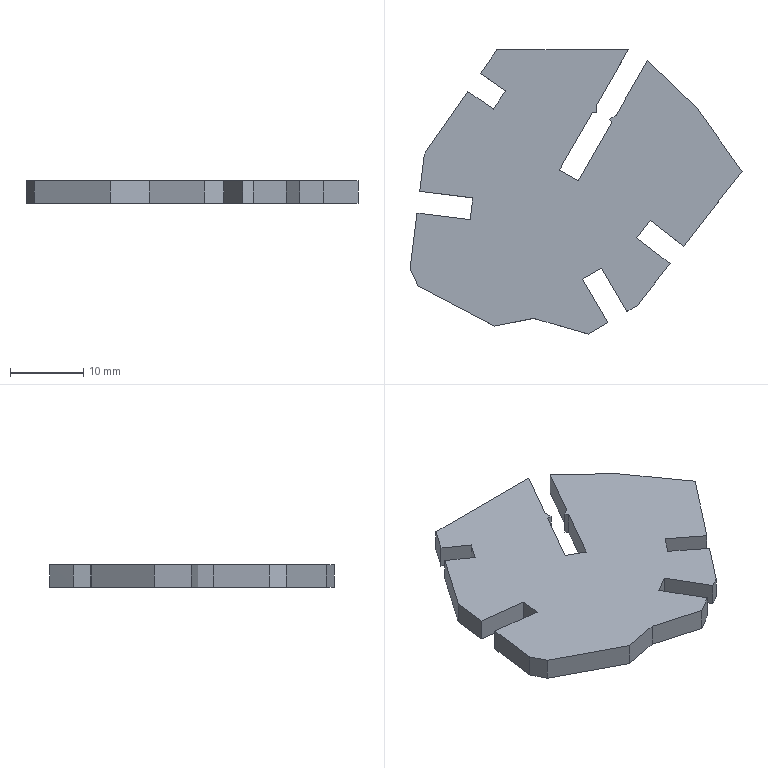Part | SolidWorks | features BaseBody 1 | 1 solid | 41 faces | box 45.246 x 38.746 x 3 mm | volume 3417 mm3 | spline 23 | plane 18